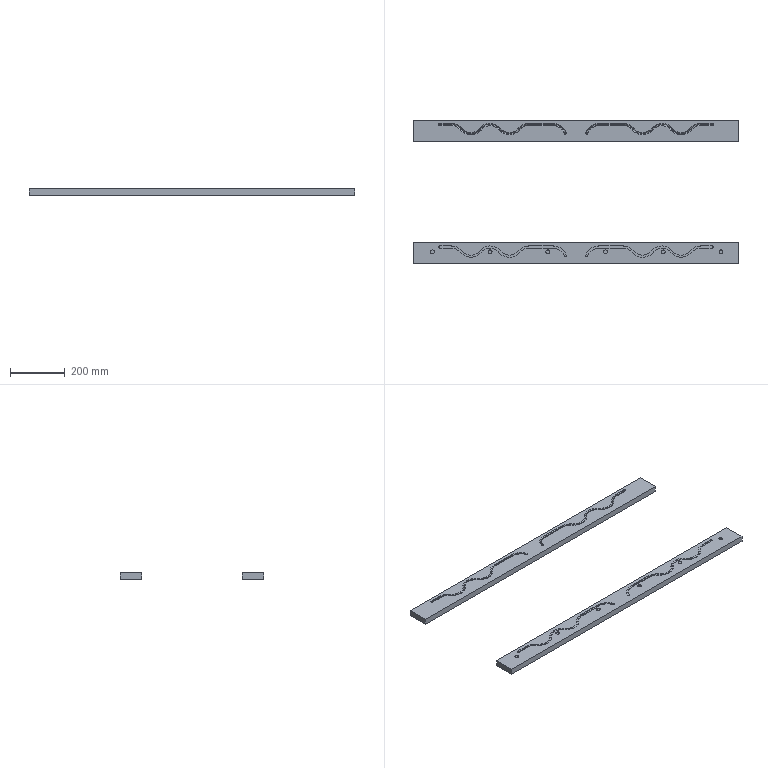NC program | NX | posted with a generic post | part box 1185 x 523.484 x 22 mm
Lines 1 to 1045 of 261559:
N10 G17 G21 G94 G90
(G81点孔 , TOOL : D6点孔钻)
N12 T01 M6
N14 /M1
N16 G54
N18 G17 G0 G90 X1050. Y5. S1500 M3
N20 G43 Z50. H1
N22 G94 G81 G98 Z-1.5 F120. R1.5
N24 X840.
N26 X630.
N28 X420.
N30 X210.
N32 X0.
N34 G80
N36 G0 X0. Y5. Z50.
N38 M5
(G83钻孔 , TOOL : Z10.3钻头)
N40 T10 M6
N42 /M1
N44 G54
N46 G17 G0 G90 X1050. Y5. S800 M3
N48 G43 Z50. H10
N50 G94 G83 G98 Z-20. F80. Q2. R1.5
N52 X840.
N54 X630.
N56 X420.
N58 X210.
N60 X0.
N62 G80
N64 G0 X0. Y5. Z50.
N66 M5
(G83钻孔_1 , TOOL : Z4.2钻头)
N68 T03 M6
N70 /M1
N72 G54
N74 G17 G0 G90 X70. Y22.5 S1000 M3
N76 G43 Z50. H3
N78 G94 G83 G98 Z-5. F20. Q2. R1.5
N80 X388.
N82 X658.
N84 X975.
N86 G80
N88 G0 X975. Y22.5 Z50.
N90 M5
(PLANAR_PROFILE , TOOL : R2球刀)
N92 T14 M6
N94 G54
N96 G17 G0 G90 X1018. Y22.5 S3000 M3
N98 G43 Z50. H14
N100 Z3.2
N102 G94 G1 Z0.1 F2000.
N104 X975.
N106 G3 X940.874 Y6.833 R45.
N108 G2 X870.874 Y4.667 R45.
N110 G3 X800.874 Y6.833 R45.
N112 G2 X730.874 Y4.667 R45.
N114 G3 X695. Y22.5 R45.
N116 G1 X605.
N118 G3 X562.073 Y-9. R45.
N120 G1 Z3.1
N122 G0 Z50.
N124 Z3.1
N126 G1 Z0.
N128 G2 X605. Y22.5 R45.
N130 G1 X695.
N132 G2 X730.874 Y4.667 R45.
N134 G3 X800.874 Y6.833 R45.
N136 G2 X870.874 Y4.667 R45.
N138 G3 X940.874 Y6.833 R45.
N140 G2 X975. Y22.5 R45.
N142 G1 X1018.
N144 Z3.
N146 G0 Z50.
N148 Z3.
N150 G1 Z-0.1
N152 X975.
N154 G3 X940.874 Y6.833 R45.
N156 G2 X870.874 Y4.667 R45.
N158 G3 X800.874 Y6.833 R45.
N160 G2 X730.874 Y4.667 R45.
N162 G3 X695. Y22.5 R45.
N164 G1 X605.
N166 G3 X562.073 Y-9. R45.
N168 G1 Z2.9
N170 G0 Z50.
N172 Z2.9
N174 G1 Z-0.2
N176 G2 X605. Y22.5 R45.
N178 G1 X695.
N180 G2 X730.874 Y4.667 R45.
N182 G3 X800.874 Y6.833 R45.
N184 G2 X870.874 Y4.667 R45.
N186 G3 X940.874 Y6.833 R45.
N188 G2 X975. Y22.5 R45.
N190 G1 X1018.
N192 Z2.8
N194 G0 Z50.
N196 Z2.8
N198 G1 Z-0.3
N200 X975.
N202 G3 X940.874 Y6.833 R45.
N204 G2 X870.874 Y4.667 R45.
N206 G3 X800.874 Y6.833 R45.
N208 G2 X730.874 Y4.667 R45.
N210 G3 X695. Y22.5 R45.
N212 G1 X605.
N214 G3 X562.073 Y-9. R45.
N216 G1 Z2.7
N218 G0 Z50.
N220 Z2.7
N222 G1 Z-0.4
N224 G2 X605. Y22.5 R45.
N226 G1 X695.
N228 G2 X730.874 Y4.667 R45.
N230 G3 X800.874 Y6.833 R45.
N232 G2 X870.874 Y4.667 R45.
N234 G3 X940.874 Y6.833 R45.
N236 G2 X975. Y22.5 R45.
N238 G1 X1018.
N240 Z2.6
N242 G0 Z50.
N244 Z2.6
N246 G1 Z-0.5
N248 X975.
N250 G3 X940.874 Y6.833 R45.
N252 G2 X870.874 Y4.667 R45.
N254 G3 X800.874 Y6.833 R45.
N256 G2 X730.874 Y4.667 R45.
N258 G3 X695. Y22.5 R45.
N260 G1 X605.
N262 G3 X562.073 Y-9. R45.
N264 G1 Z2.5
N266 G0 Z50.
N268 Z2.5
N270 G1 Z-0.6
N272 G2 X605. Y22.5 R45.
N274 G1 X695.
N276 G2 X730.874 Y4.667 R45.
N278 G3 X800.874 Y6.833 R45.
N280 G2 X870.874 Y4.667 R45.
N282 G3 X940.874 Y6.833 R45.
N284 G2 X975. Y22.5 R45.
N286 G1 X1018.
N288 Z2.4
N290 G0 Z50.
N292 Z2.4
N294 G1 Z-0.7
N296 X975.
N298 G3 X940.874 Y6.833 R45.
N300 G2 X870.874 Y4.667 R45.
N302 G3 X800.874 Y6.833 R45.
N304 G2 X730.874 Y4.667 R45.
N306 G3 X695. Y22.5 R45.
N308 G1 X605.
N310 G3 X562.073 Y-9. R45.
N312 G1 Z2.3
N314 G0 Z50.
N316 Z2.3
N318 G1 Z-0.8
N320 G2 X605. Y22.5 R45.
N322 G1 X695.
N324 G2 X730.874 Y4.667 R45.
N326 G3 X800.874 Y6.833 R45.
N328 G2 X870.874 Y4.667 R45.
N330 G3 X940.874 Y6.833 R45.
N332 G2 X975. Y22.5 R45.
N334 G1 X1018.
N336 Z2.2
N338 G0 Z50.
N340 Z2.2
N342 G1 Z-0.9
N344 X975.
N346 G3 X940.874 Y6.833 R45.
N348 G2 X870.874 Y4.667 R45.
N350 G3 X800.874 Y6.833 R45.
N352 G2 X730.874 Y4.667 R45.
N354 G3 X695. Y22.5 R45.
N356 G1 X605.
N358 G3 X562.073 Y-9. R45.
N360 G1 Z2.1
N362 G0 Z50.
N364 Z2.1
N366 G1 Z-1.
N368 G2 X605. Y22.5 R45.
N370 G1 X695.
N372 G2 X730.874 Y4.667 R45.
N374 G3 X800.874 Y6.833 R45.
N376 G2 X870.874 Y4.667 R45.
N378 G3 X940.874 Y6.833 R45.
N380 G2 X975. Y22.5 R45.
N382 G1 X1018.
N384 Z2.
N386 G0 Z50.
N388 Z2.
N390 G1 Z-1.1
N392 X975.
N394 G3 X940.874 Y6.833 R45.
N396 G2 X870.874 Y4.667 R45.
N398 G3 X800.874 Y6.833 R45.
N400 G2 X730.874 Y4.667 R45.
N402 G3 X695. Y22.5 R45.
N404 G1 X605.
N406 G3 X562.073 Y-9. R45.
N408 G1 Z1.9
N410 G0 Z50.
N412 Z1.9
N414 G1 Z-1.2
N416 G2 X605. Y22.5 R45.
N418 G1 X695.
N420 G2 X730.874 Y4.667 R45.
N422 G3 X800.874 Y6.833 R45.
N424 G2 X870.874 Y4.667 R45.
N426 G3 X940.874 Y6.833 R45.
N428 G2 X975. Y22.5 R45.
N430 G1 X1018.
N432 Z1.8
N434 G0 Z50.
N436 Z1.8
N438 G1 Z-1.3
N440 X975.
N442 G3 X940.874 Y6.833 R45.
N444 G2 X870.874 Y4.667 R45.
N446 G3 X800.874 Y6.833 R45.
N448 G2 X730.874 Y4.667 R45.
N450 G3 X695. Y22.5 R45.
N452 G1 X605.
N454 G3 X562.073 Y-9. R45.
N456 G1 Z1.7
N458 G0 Z50.
N460 Z1.7
N462 G1 Z-1.4
N464 G2 X605. Y22.5 R45.
N466 G1 X695.
N468 G2 X730.874 Y4.667 R45.
N470 G3 X800.874 Y6.833 R45.
N472 G2 X870.874 Y4.667 R45.
N474 G3 X940.874 Y6.833 R45.
N476 G2 X975. Y22.5 R45.
N478 G1 X1018.
N480 Z1.6
N482 G0 Z50.
N484 Z1.6
N486 G1 Z-1.5
N488 X975.
N490 G3 X940.874 Y6.833 R45.
N492 G2 X870.874 Y4.667 R45.
N494 G3 X800.874 Y6.833 R45.
N496 G2 X730.874 Y4.667 R45.
N498 G3 X695. Y22.5 R45.
N500 G1 X605.
N502 G3 X562.073 Y-9. R45.
N504 G1 Z1.5
N506 G0 Z50.
N508 Z1.5
N510 G1 Z-1.6
N512 G2 X605. Y22.5 R45.
N514 G1 X695.
N516 G2 X730.874 Y4.667 R45.
N518 G3 X800.874 Y6.833 R45.
N520 G2 X870.874 Y4.667 R45.
N522 G3 X940.874 Y6.833 R45.
N524 G2 X975. Y22.5 R45.
N526 G1 X1018.
N528 Z1.4
N530 G0 Z50.
N532 Z1.4
N534 G1 Z-1.7
N536 X975.
N538 G3 X940.874 Y6.833 R45.
N540 G2 X870.874 Y4.667 R45.
N542 G3 X800.874 Y6.833 R45.
N544 G2 X730.874 Y4.667 R45.
N546 G3 X695. Y22.5 R45.
N548 G1 X605.
N550 G3 X562.073 Y-9. R45.
N552 G1 Z1.3
N554 G0 Z50.
N556 Z1.3
N558 G1 Z-1.8
N560 G2 X605. Y22.5 R45.
N562 G1 X695.
N564 G2 X730.874 Y4.667 R45.
N566 G3 X800.874 Y6.833 R45.
N568 G2 X870.874 Y4.667 R45.
N570 G3 X940.874 Y6.833 R45.
N572 G2 X975. Y22.5 R45.
N574 G1 X1018.
N576 Z1.2
N578 G0 Z50.
N580 Z1.2
N582 G1 Z-1.9
N584 X975.
N586 G3 X940.874 Y6.833 R45.
N588 G2 X870.874 Y4.667 R45.
N590 G3 X800.874 Y6.833 R45.
N592 G2 X730.874 Y4.667 R45.
N594 G3 X695. Y22.5 R45.
N596 G1 X605.
N598 G3 X562.073 Y-9. R45.
N600 G1 Z1.1
N602 G0 Z50.
N604 Z1.1
N606 G1 Z-2.
N608 G2 X605. Y22.5 R45.
N610 G1 X695.
N612 G2 X730.874 Y4.667 R45.
N614 G3 X800.874 Y6.833 R45.
N616 G2 X870.874 Y4.667 R45.
N618 G3 X940.874 Y6.833 R45.
N620 G2 X975. Y22.5 R45.
N622 G1 X1018.
N624 Z1.
N626 G0 Z50.
N628 Z1.
N630 G1 Z-2.1
N632 X975.
N634 G3 X940.874 Y6.833 R45.
N636 G2 X870.874 Y4.667 R45.
N638 G3 X800.874 Y6.833 R45.
N640 G2 X730.874 Y4.667 R45.
N642 G3 X695. Y22.5 R45.
N644 G1 X605.
N646 G3 X562.073 Y-9. R45.
N648 G1 Z0.9
N650 G0 Z50.
N652 Z0.9
N654 G1 Z-2.2
N656 G2 X605. Y22.5 R45.
N658 G1 X695.
N660 G2 X730.874 Y4.667 R45.
N662 G3 X800.874 Y6.833 R45.
N664 G2 X870.874 Y4.667 R45.
N666 G3 X940.874 Y6.833 R45.
N668 G2 X975. Y22.5 R45.
N670 G1 X1018.
N672 Z0.8
N674 G0 Z50.
N676 Z0.8
N678 G1 Z-2.3
N680 X975.
N682 G3 X940.874 Y6.833 R45.
N684 G2 X870.874 Y4.667 R45.
N686 G3 X800.874 Y6.833 R45.
N688 G2 X730.874 Y4.667 R45.
N690 G3 X695. Y22.5 R45.
N692 G1 X605.
N694 G3 X562.073 Y-9. R45.
N696 G1 Z0.7
N698 G0 Z50.
N700 Z0.7
N702 G1 Z-2.4
N704 G2 X605. Y22.5 R45.
N706 G1 X695.
N708 G2 X730.874 Y4.667 R45.
N710 G3 X800.874 Y6.833 R45.
N712 G2 X870.874 Y4.667 R45.
N714 G3 X940.874 Y6.833 R45.
N716 G2 X975. Y22.5 R45.
N718 G1 X1018.
N720 Z0.6
N722 G0 Z50.
N724 Z0.6
N726 G1 Z-2.5
N728 X975.
N730 G3 X940.874 Y6.833 R45.
N732 G2 X870.874 Y4.667 R45.
N734 G3 X800.874 Y6.833 R45.
N736 G2 X730.874 Y4.667 R45.
N738 G3 X695. Y22.5 R45.
N740 G1 X605.
N742 G3 X562.073 Y-9. R45.
N744 G1 Z0.5
N746 G0 Z50.
N748 Z0.5
N750 G1 Z-2.6
N752 G2 X605. Y22.5 R45.
N754 G1 X695.
N756 G2 X730.874 Y4.667 R45.
N758 G3 X800.874 Y6.833 R45.
N760 G2 X870.874 Y4.667 R45.
N762 G3 X940.874 Y6.833 R45.
N764 G2 X975. Y22.5 R45.
N766 G1 X1018.
N768 Z0.4
N770 G0 Z50.
N772 Z0.4
N774 G1 Z-2.7
N776 X975.
N778 G3 X940.874 Y6.833 R45.
N780 G2 X870.874 Y4.667 R45.
N782 G3 X800.874 Y6.833 R45.
N784 G2 X730.874 Y4.667 R45.
N786 G3 X695. Y22.5 R45.
N788 G1 X605.
N790 G3 X562.073 Y-9. R45.
N792 G1 Z0.3
N794 G0 Z50.
N796 Z0.3
N798 G1 Z-2.8
N800 G2 X605. Y22.5 R45.
N802 G1 X695.
N804 G2 X730.874 Y4.667 R45.
N806 G3 X800.874 Y6.833 R45.
N808 G2 X870.874 Y4.667 R45.
N810 G3 X940.874 Y6.833 R45.
N812 G2 X975. Y22.5 R45.
N814 G1 X1018.
N816 Z0.2
N818 G0 Z50.
N820 Z0.2
N822 G1 Z-2.9
N824 X975.
N826 G3 X940.874 Y6.833 R45.
N828 G2 X870.874 Y4.667 R45.
N830 G3 X800.874 Y6.833 R45.
N832 G2 X730.874 Y4.667 R45.
N834 G3 X695. Y22.5 R45.
N836 G1 X605.
N838 G3 X562.073 Y-9. R45.
N840 G1 Z0.1
N842 G0 Z50.
N844 Z0.1
N846 G1 Z-3.
N848 G2 X605. Y22.5 R45.
N850 G1 X695.
N852 G2 X730.874 Y4.667 R45.
N854 G3 X800.874 Y6.833 R45.
N856 G2 X870.874 Y4.667 R45.
N858 G3 X940.874 Y6.833 R45.
N860 G2 X975. Y22.5 R45.
N862 G1 X1018.
N864 Z0.
N866 G0 Z50.
N868 Z0.
N870 G1 Z-3.1
N872 X975.
N874 G3 X940.874 Y6.833 R45.
N876 G2 X870.874 Y4.667 R45.
N878 G3 X800.874 Y6.833 R45.
N880 G2 X730.874 Y4.667 R45.
N882 G3 X695. Y22.5 R45.
N884 G1 X605.
N886 G3 X562.073 Y-9. R45.
N888 G1 Z-0.1
N890 G0 Z50.
N892 Z-0.1
N894 G1 Z-3.2
N896 G2 X605. Y22.5 R45.
N898 G1 X695.
N900 G2 X730.874 Y4.667 R45.
N902 G3 X800.874 Y6.833 R45.
N904 G2 X870.874 Y4.667 R45.
N906 G3 X940.874 Y6.833 R45.
N908 G2 X975. Y22.5 R45.
N910 G1 X1018.
N912 Z-0.2
N914 G0 Z50.
N916 Z-0.2
N918 G1 Z-3.3
N920 X975.
N922 G3 X940.874 Y6.833 R45.
N924 G2 X870.874 Y4.667 R45.
N926 G3 X800.874 Y6.833 R45.
N928 G2 X730.874 Y4.667 R45.
N930 G3 X695. Y22.5 R45.
N932 G1 X605.
N934 G3 X562.073 Y-9. R45.
N936 G1 Z-0.3
N938 G0 Z50.
N940 Z-0.3
N942 G1 Z-3.4
N944 G2 X605. Y22.5 R45.
N946 G1 X695.
N948 G2 X730.874 Y4.667 R45.
N950 G3 X800.874 Y6.833 R45.
N952 G2 X870.874 Y4.667 R45.
N954 G3 X940.874 Y6.833 R45.
N956 G2 X975. Y22.5 R45.
N958 G1 X1018.
N960 Z-0.4
N962 G0 Z50.
N964 Z-0.4
N966 G1 Z-3.5
N968 X975.
N970 G3 X940.874 Y6.833 R45.
N972 G2 X870.874 Y4.667 R45.
N974 G3 X800.874 Y6.833 R45.
N976 G2 X730.874 Y4.667 R45.
N978 G3 X695. Y22.5 R45.
N980 G1 X605.
N982 G3 X562.073 Y-9. R45.
N984 G1 Z-0.5
N986 G0 Z50.
N988 Z-0.5
N990 G1 Z-3.6
N992 G2 X605. Y22.5 R45.
N994 G1 X695.
N996 G2 X730.874 Y4.667 R45.
N998 G3 X800.874 Y6.833 R45.
N1000 G2 X870.874 Y4.667 R45.
N1002 G3 X940.874 Y6.833 R45.
N1004 G2 X975. Y22.5 R45.
N1006 G1 X1018.
N1008 Z-0.6
N1010 G0 Z50.
N1012 Z-0.6
N1014 G1 Z-3.7
N1016 X975.
N1018 G3 X940.874 Y6.833 R45.
N1020 G2 X870.874 Y4.667 R45.
N1022 G3 X800.874 Y6.833 R45.
N1024 G2 X730.874 Y4.667 R45.
N1026 G3 X695. Y22.5 R45.
N1028 G1 X605.
N1030 G3 X562.073 Y-9. R45.
N1032 G1 Z-0.7
N1034 G0 Z50.
N1036 Z-0.7
N1038 G1 Z-3.8
N1040 G2 X605. Y22.5 R45.
N1042 G1 X695.
N1044 G2 X730.874 Y4.667 R45.
N1046 G3 X800.874 Y6.833 R45.
N1048 G2 X870.874 Y4.667 R45.
N1050 G3 X940.874 Y6.833 R45.
N1052 G2 X975. Y22.5 R45.
N1054 G1 X1018.
N1056 Z-0.8
N1058 G0 Z50.
N1060 Z-0.8
N1062 G1 Z-3.9
N1064 X975.
N1066 G3 X940.874 Y6.833 R45.
N1068 G2 X870.874 Y4.667 R45.
N1070 G3 X800.874 Y6.833 R45.
N1072 G2 X730.874 Y4.667 R45.
N1074 G3 X695. Y22.5 R45.
N1076 G1 X605.
N1078 G3 X562.073 Y-9. R45.
N1080 G1 Z-0.9
N1082 G0 Z50.
N1084 Z-0.9
N1086 G1 Z-4.
N1088 G2 X605. Y22.5 R45.
N1090 G1 X695.
N1092 G2 X730.874 Y4.667 R45.
N1094 G3 X800.874 Y6.833 R45.
N1096 G2 X870.874 Y4.667 R45.
N1098 G3 X940.874 Y6.833 R45.
N1100 G2 X975. Y22.5 R45.
N1102 G1 X1018.
N1104 Z-1.
N1106 G0 Z50.
N1108 X482.927 Y-9.
N1110 Z3.
N1112 G1 Z-0.1
N1114 G3 X440. Y22.5 R45.
N1116 G1 X350.
N1118 G3 X314.125 Y4.666 R45.
N1120 G2 X244.126 Y6.833 R45.
N1122 G3 X174.125 Y4.666 R45.
N1124 G2 X105.875 Y4.666 R45.
N1126 G3 X70. Y22.5 R45.
N1128 G1 X27.
N1130 Z2.9
N1132 G0 Z50.
N1134 Z2.9
N1136 G1 Z-0.2
N1138 X70.
N1140 G2 X105.875 Y4.666 R45.
N1142 G3 X174.125 Y4.666 R45.
N1144 G2 X244.126 Y6.833 R45.
N1146 G3 X314.125 Y4.666 R45.
N1148 G2 X350. Y22.5 R45.
N1150 G1 X440.
N1152 G2 X482.927 Y-9. R45.
N1154 G1 Z2.8
N1156 G0 Z50.
N1158 Z2.8
N1160 G1 Z-0.3
N1162 G3 X440. Y22.5 R45.
N1164 G1 X350.
N1166 G3 X314.125 Y4.666 R45.
N1168 G2 X244.126 Y6.833 R45.
N1170 G3 X174.125 Y4.666 R45.
N1172 G2 X105.875 Y4.666 R45.
N1174 G3 X70. Y22.5 R45.
N1176 G1 X27.
N1178 Z2.7
N1180 G0 Z50.
N1182 Z2.7
N1184 G1 Z-0.4
N1186 X70.
N1188 G2 X105.875 Y4.666 R45.
N1190 G3 X174.125 Y4.666 R45.
N1192 G2 X244.126 Y6.833 R45.
N1194 G3 X314.125 Y4.666 R45.
N1196 G2 X350. Y22.5 R45.
N1198 G1 X440.
N1200 G2 X482.927 Y-9. R45.
N1202 G1 Z2.6
N1204 G0 Z50.
N1206 Z2.6
N1208 G1 Z-0.5
N1210 G3 X440. Y22.5 R45.
N1212 G1 X350.
N1214 G3 X314.125 Y4.666 R45.
N1216 G2 X244.126 Y6.833 R45.
N1218 G3 X174.125 Y4.666 R45.
N1220 G2 X105.875 Y4.666 R45.
N1222 G3 X70. Y22.5 R45.
N1224 G1 X27.
N1226 Z2.5
N1228 G0 Z50.
N1230 Z2.5
N1232 G1 Z-0.6
N1234 X70.
N1236 G2 X105.875 Y4.666 R45.
N1238 G3 X174.125 Y4.666 R45.
N1240 G2 X244.126 Y6.833 R45.
N1242 G3 X314.125 Y4.666 R45.
N1244 G2 X350. Y22.5 R45.
N1246 G1 X440.
N1248 G2 X482.927 Y-9. R45.
N1250 G1 Z2.4
N1252 G0 Z50.
N1254 Z2.4
N1256 G1 Z-0.7
N1258 G3 X440. Y22.5 R45.
N1260 G1 X350.
N1262 G3 X314.125 Y4.666 R45.
N1264 G2 X244.126 Y6.833 R45.
N1266 G3 X174.125 Y4.666 R45.
N1268 G2 X105.875 Y4.666 R45.
N1270 G3 X70. Y22.5 R45.
N1272 G1 X27.
N1274 Z2.3
N1276 G0 Z50.
N1278 Z2.3
N1280 G1 Z-0.8
N1282 X70.
N1284 G2 X105.875 Y4.666 R45.
N1286 G3 X174.125 Y4.666 R45.
N1288 G2 X244.126 Y6.833 R45.
N1290 G3 X314.125 Y4.666 R45.
N1292 G2 X350. Y22.5 R45.
N1294 G1 X440.
N1296 G2 X482.927 Y-9. R45.
N1298 G1 Z2.2
N1300 G0 Z50.
N1302 Z2.2
N1304 G1 Z-0.9
N1306 G3 X440. Y22.5 R45.
N1308 G1 X350.
N1310 G3 X314.125 Y4.666 R45.
N1312 G2 X244.126 Y6.833 R45.
N1314 G3 X174.125 Y4.666 R45.
N1316 G2 X105.875 Y4.666 R45.
N1318 G3 X70. Y22.5 R45.
N1320 G1 X27.
N1322 Z2.1
N1324 G0 Z50.
N1326 Z2.1
N1328 G1 Z-1.
N1330 X70.
N1332 G2 X105.875 Y4.666 R45.
N1334 G3 X174.125 Y4.666 R45.
N1336 G2 X244.126 Y6.833 R45.
N1338 G3 X314.125 Y4.666 R45.
N1340 G2 X350. Y22.5 R45.
N1342 G1 X440.
N1344 G2 X482.927 Y-9. R45.
N1346 G1 Z2.
N1348 G0 Z50.
N1350 Z2.
N1352 G1 Z-1.1
N1354 G3 X440. Y22.5 R45.
N1356 G1 X350.
N1358 G3 X314.125 Y4.666 R45.
N1360 G2 X244.126 Y6.833 R45.
N1362 G3 X174.125 Y4.666 R45.
N1364 G2 X105.875 Y4.666 R45.
N1366 G3 X70. Y22.5 R45.
N1368 G1 X27.
N1370 Z1.9
N1372 G0 Z50.
N1374 Z1.9
N1376 G1 Z-1.2
N1378 X70.
N1380 G2 X105.875 Y4.666 R45.
N1382 G3 X174.125 Y4.666 R45.
N1384 G2 X244.126 Y6.833 R45.
N1386 G3 X314.125 Y4.666 R45.
N1388 G2 X350. Y22.5 R45.
N1390 G1 X440.
N1392 G2 X482.927 Y-9. R45.
N1394 G1 Z1.8
N1396 G0 Z50.
N1398 Z1.8
N1400 G1 Z-1.3
N1402 G3 X440. Y22.5 R45.
N1404 G1 X350.
N1406 G3 X314.125 Y4.666 R45.
N1408 G2 X244.126 Y6.833 R45.
N1410 G3 X174.125 Y4.666 R45.
N1412 G2 X105.875 Y4.666 R45.
N1414 G3 X70. Y22.5 R45.
N1416 G1 X27.
N1418 Z1.7
N1420 G0 Z50.
N1422 Z1.7
N1424 G1 Z-1.4
N1426 X70.
N1428 G2 X105.875 Y4.666 R45.
N1430 G3 X174.125 Y4.666 R45.
N1432 G2 X244.126 Y6.833 R45.
N1434 G3 X314.125 Y4.666 R45.
N1436 G2 X350. Y22.5 R45.
N1438 G1 X440.
N1440 G2 X482.927 Y-9. R45.
N1442 G1 Z1.6
N1444 G0 Z50.
N1446 Z1.6
N1448 G1 Z-1.5
N1450 G3 X440. Y22.5 R45.
N1452 G1 X350.
N1454 G3 X314.125 Y4.666 R45.
N1456 G2 X244.126 Y6.833 R45.
N1458 G3 X174.125 Y4.666 R45.
N1460 G2 X105.875 Y4.666 R45.
N1462 G3 X70. Y22.5 R45.
N1464 G1 X27.
N1466 Z1.5
N1468 G0 Z50.
N1470 Z1.5
N1472 G1 Z-1.6
N1474 X70.
N1476 G2 X105.875 Y4.666 R45.
N1478 G3 X174.125 Y4.666 R45.
N1480 G2 X244.126 Y6.833 R45.
N1482 G3 X314.125 Y4.666 R45.
N1484 G2 X350. Y22.5 R45.
N1486 G1 X440.
N1488 G2 X482.927 Y-9. R45.
N1490 G1 Z1.4
N1492 G0 Z50.
N1494 Z1.4
N1496 G1 Z-1.7
N1498 G3 X440. Y22.5 R45.
N1500 G1 X350.
N1502 G3 X314.125 Y4.666 R45.
N1504 G2 X244.126 Y6.833 R45.
N1506 G3 X174.125 Y4.666 R45.
N1508 G2 X105.875 Y4.666 R45.
N1510 G3 X70. Y22.5 R45.
N1512 G1 X27.
N1514 Z1.3
N1516 G0 Z50.
N1518 Z1.3
N1520 G1 Z-1.8
N1522 X70.
N1524 G2 X105.875 Y4.666 R45.
N1526 G3 X174.125 Y4.666 R45.
N1528 G2 X244.126 Y6.833 R45.
N1530 G3 X314.125 Y4.666 R45.
N1532 G2 X350. Y22.5 R45.
N1534 G1 X440.
N1536 G2 X482.927 Y-9. R45.
N1538 G1 Z1.2
N1540 G0 Z50.
N1542 Z1.2
N1544 G1 Z-1.9
N1546 G3 X440. Y22.5 R45.
N1548 G1 X350.
N1550 G3 X314.125 Y4.666 R45.
N1552 G2 X244.126 Y6.833 R45.
N1554 G3 X174.125 Y4.666 R45.
N1556 G2 X105.875 Y4.666 R45.
N1558 G3 X70. Y22.5 R45.
N1560 G1 X27.
N1562 Z1.1
N1564 G0 Z50.
N1566 Z1.1
N1568 G1 Z-2.
N1570 X70.
N1572 G2 X105.875 Y4.666 R45.
N1574 G3 X174.125 Y4.666 R45.
N1576 G2 X244.126 Y6.833 R45.
N1578 G3 X314.125 Y4.666 R45.
N1580 G2 X350. Y22.5 R45.
N1582 G1 X440.
N1584 G2 X482.927 Y-9. R45.
N1586 G1 Z1.
N1588 G0 Z50.
N1590 Z1.
N1592 G1 Z-2.1
N1594 G3 X440. Y22.5 R45.
N1596 G1 X350.
N1598 G3 X314.125 Y4.666 R45.
N1600 G2 X244.126 Y6.833 R45.
N1602 G3 X174.125 Y4.666 R45.
N1604 G2 X105.875 Y4.666 R45.
N1606 G3 X70. Y22.5 R45.
N1608 G1 X27.
N1610 Z0.9
N1612 G0 Z50.
N1614 Z0.9
N1616 G1 Z-2.2
N1618 X70.
N1620 G2 X105.875 Y4.666 R45.
N1622 G3 X174.125 Y4.666 R45.
N1624 G2 X244.126 Y6.833 R45.
N1626 G3 X314.125 Y4.666 R45.
N1628 G2 X350. Y22.5 R45.
N1630 G1 X440.
N1632 G2 X482.927 Y-9. R45.
N1634 G1 Z0.8
N1636 G0 Z50.
N1638 Z0.8
N1640 G1 Z-2.3
N1642 G3 X440. Y22.5 R45.
N1644 G1 X350.
N1646 G3 X314.125 Y4.666 R45.
N1648 G2 X244.126 Y6.833 R45.
N1650 G3 X174.125 Y4.666 R45.
N1652 G2 X105.875 Y4.666 R45.
N1654 G3 X70. Y22.5 R45.
N1656 G1 X27.
N1658 Z0.7
N1660 G0 Z50.
N1662 Z0.7
N1664 G1 Z-2.4
N1666 X70.
N1668 G2 X105.875 Y4.666 R45.
N1670 G3 X174.125 Y4.666 R45.
N1672 G2 X244.126 Y6.833 R45.
N1674 G3 X314.125 Y4.666 R45.
N1676 G2 X350. Y22.5 R45.
N1678 G1 X440.
N1680 G2 X482.927 Y-9. R45.
N1682 G1 Z0.6
N1684 G0 Z50.
N1686 Z0.6
N1688 G1 Z-2.5
N1690 G3 X440. Y22.5 R45.
N1692 G1 X350.
N1694 G3 X314.125 Y4.666 R45.
N1696 G2 X244.126 Y6.833 R45.
N1698 G3 X174.125 Y4.666 R45.
N1700 G2 X105.875 Y4.666 R45.
N1702 G3 X70. Y22.5 R45.
N1704 G1 X27.
N1706 Z0.5
N1708 G0 Z50.
N1710 Z0.5
N1712 G1 Z-2.6
N1714 X70.
N1716 G2 X105.875 Y4.666 R45.
N1718 G3 X174.125 Y4.666 R45.
N1720 G2 X244.126 Y6.833 R45.
N1722 G3 X314.125 Y4.666 R45.
N1724 G2 X350. Y22.5 R45.
N1726 G1 X440.
N1728 G2 X482.927 Y-9. R45.
N1730 G1 Z0.4
N1732 G0 Z50.
N1734 Z0.4
N1736 G1 Z-2.7
N1738 G3 X440. Y22.5 R45.
N1740 G1 X350.
N1742 G3 X314.125 Y4.666 R45.
N1744 G2 X244.126 Y6.833 R45.
N1746 G3 X174.125 Y4.666 R45.
N1748 G2 X105.875 Y4.666 R45.
N1750 G3 X70. Y22.5 R45.
N1752 G1 X27.
N1754 Z0.3
N1756 G0 Z50.
N1758 Z0.3
N1760 G1 Z-2.8
N1762 X70.
N1764 G2 X105.875 Y4.666 R45.
N1766 G3 X174.125 Y4.666 R45.
N1768 G2 X244.126 Y6.833 R45.
N1770 G3 X314.125 Y4.666 R45.
N1772 G2 X350. Y22.5 R45.
N1774 G1 X440.
N1776 G2 X482.927 Y-9. R45.
N1778 G1 Z0.2
N1780 G0 Z50.
N1782 Z0.2
N1784 G1 Z-2.9
N1786 G3 X440. Y22.5 R45.
N1788 G1 X350.
N1790 G3 X314.125 Y4.666 R45.
N1792 G2 X244.126 Y6.833 R45.
N1794 G3 X174.125 Y4.666 R45.
N1796 G2 X105.875 Y4.666 R45.
N1798 G3 X70. Y22.5 R45.
N1800 G1 X27.
N1802 Z0.1
N1804 G0 Z50.
N1806 Z0.1
N1808 G1 Z-3.
N1810 X70.
N1812 G2 X105.875 Y4.666 R45.
N1814 G3 X174.125 Y4.666 R45.
N1816 G2 X244.126 Y6.833 R45.
N1818 G3 X314.125 Y4.666 R45.
N1820 G2 X350. Y22.5 R45.
N1822 G1 X440.
N1824 G2 X482.927 Y-9. R45.
N1826 G1 Z0.
N1828 G0 Z50.
N1830 Z0.
N1832 G1 Z-3.1
N1834 G3 X440. Y22.5 R45.
N1836 G1 X350.
N1838 G3 X314.125 Y4.666 R45.
N1840 G2 X244.126 Y6.833 R45.
N1842 G3 X174.125 Y4.666 R45.
N1844 G2 X105.875 Y4.666 R45.
N1846 G3 X70. Y22.5 R45.
N1848 G1 X27.
N1850 Z-0.1
N1852 G0 Z50.
N1854 Z-0.1
N1856 G1 Z-3.2
N1858 X70.
N1860 G2 X105.875 Y4.666 R45.
N1862 G3 X174.125 Y4.666 R45.
N1864 G2 X244.126 Y6.833 R45.
N1866 G3 X314.125 Y4.666 R45.
N1868 G2 X350. Y22.5 R45.
N1870 G1 X440.
N1872 G2 X482.927 Y-9. R45.
N1874 G1 Z-0.2
N1876 G0 Z50.
N1878 Z-0.2
N1880 G1 Z-3.3
N1882 G3 X440. Y22.5 R45.
N1884 G1 X350.
N1886 G3 X314.125 Y4.666 R45.
N1888 G2 X244.126 Y6.833 R45.
N1890 G3 X174.125 Y4.666 R45.
N1892 G2 X105.875 Y4.666 R45.
N1894 G3 X70. Y22.5 R45.
N1896 G1 X27.
N1898 Z-0.3
N1900 G0 Z50.
N1902 Z-0.3
N1904 G1 Z-3.4
N1906 X70.
N1908 G2 X105.875 Y4.666 R45.
N1910 G3 X174.125 Y4.666 R45.
N1912 G2 X244.126 Y6.833 R45.
N1914 G3 X314.125 Y4.666 R45.
N1916 G2 X350. Y22.5 R45.
N1918 G1 X440.
N1920 G2 X482.927 Y-9. R45.
N1922 G1 Z-0.4
N1924 G0 Z50.
N1926 Z-0.4
N1928 G1 Z-3.5
N1930 G3 X440. Y22.5 R45.
N1932 G1 X350.
N1934 G3 X314.125 Y4.666 R45.
N1936 G2 X244.126 Y6.833 R45.
N1938 G3 X174.125 Y4.666 R45.
N1940 G2 X105.875 Y4.666 R45.
N1942 G3 X70. Y22.5 R45.
N1944 G1 X27.
N1946 Z-0.5
N1948 G0 Z50.
N1950 Z-0.5
N1952 G1 Z-3.6
N1954 X70.
N1956 G2 X105.875 Y4.666 R45.
N1958 G3 X174.125 Y4.666 R45.
N1960 G2 X244.126 Y6.833 R45.
N1962 G3 X314.125 Y4.666 R45.
N1964 G2 X350. Y22.5 R45.
N1966 G1 X440.
N1968 G2 X482.927 Y-9. R45.
N1970 G1 Z-0.6
N1972 G0 Z50.
N1974 Z-0.6
N1976 G1 Z-3.7
N1978 G3 X440. Y22.5 R45.
N1980 G1 X350.
N1982 G3 X314.125 Y4.666 R45.
N1984 G2 X244.126 Y6.833 R45.
N1986 G3 X174.125 Y4.666 R45.
N1988 G2 X105.875 Y4.666 R45.
N1990 G3 X70. Y22.5 R45.
N1992 G1 X27.
N1994 Z-0.7
N1996 G0 Z50.
N1998 Z-0.7
N2000 G1 Z-3.8
N2002 X70.
N2004 G2 X105.875 Y4.666 R45.
N2006 G3 X174.125 Y4.666 R45.
N2008 G2 X244.126 Y6.833 R45.
N2010 G3 X314.125 Y4.666 R45.
N2012 G2 X350. Y22.5 R45.
N2014 G1 X440.
N2016 G2 X482.927 Y-9. R45.
N2018 G1 Z-0.8
N2020 G0 Z50.
N2022 Z-0.8
N2024 G1 Z-3.9
N2026 G3 X440. Y22.5 R45.
N2028 G1 X350.
N2030 G3 X314.125 Y4.666 R45.
N2032 G2 X244.126 Y6.833 R45.
N2034 G3 X174.125 Y4.666 R45.
N2036 G2 X105.875 Y4.666 R45.
N2038 G3 X70. Y22.5 R45.
N2040 G1 X27.
N2042 Z-0.9
N2044 G0 Z50.
N2046 Z-0.9
N2048 G1 Z-4.
N2050 X70.
N2052 G2 X105.875 Y4.666 R45.
N2054 G3 X174.125 Y4.666 R45.
N2056 G2 X244.126 Y6.833 R45.
N2058 G3 X314.125 Y4.666 R45.
N2060 G2 X350. Y22.5 R45.
N2062 G1 X440.
N2064 G2 X482.927 Y-9. R45.
N2066 G1 Z-1.
N2068 G0 Z50.
N2070 M5